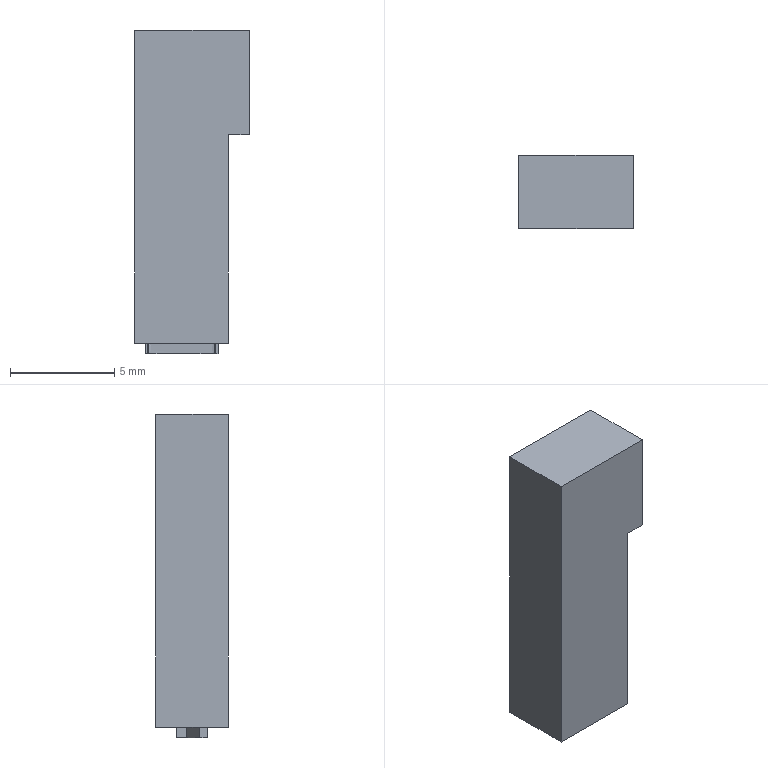Part | STEP file | gslz 2016.10.28-10_id1650_x_t | 1 solid | 31 faces | box 5.5 x 3.5 x 15.5 mm | volume 254.405 mm3 | plane 22 | other 9